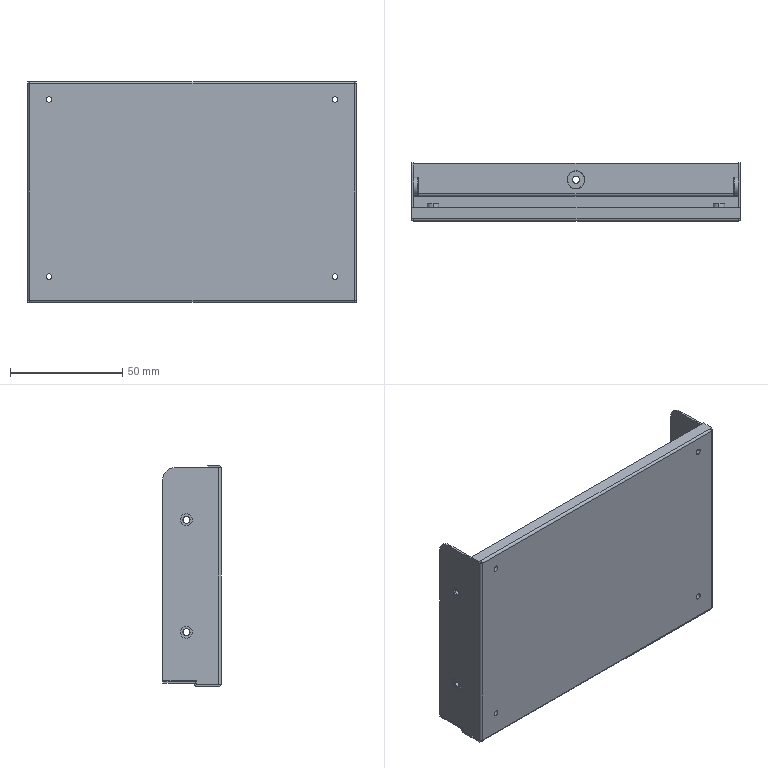Part | SolidWorks | features BaseBody 6 | 6 solids | 137 faces | box 146.9 x 26 x 98.5 mm | volume 19821 mm3 | cylinder 70 | plane 57 | spline 10 | commonest cylinder face diameters 3 x10 3.3 x10 5.4 x10 8 x10 2.5 x8 5 x8